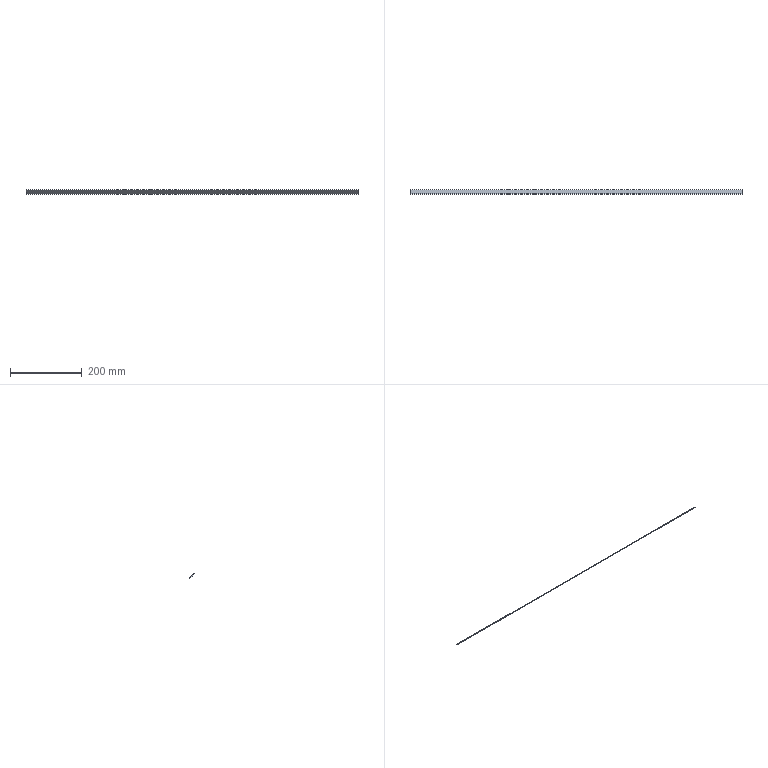Part | SolidWorks | features BaseBody 1 | 1 solid | 6 faces | box 924.6 x 13.8 x 13.8 mm | volume 24987 mm3 | plane 6
STEP:
#1=CARTESIAN_POINT('',(924.6,13.8,2.121));
#2=VERTEX_POINT('',#1);
#3=CARTESIAN_POINT('',(924.6,13.8,0.));
#4=VERTEX_POINT('',#3);
#5=CARTESIAN_POINT('',(924.6,13.8,0.));
#6=DIRECTION('',(0.,0.,-1.));
#7=VECTOR('',#6,1000.);
#8=LINE('',#5,#7);
#9=EDGE_CURVE('',#2,#4,#8,.T.);
#10=ORIENTED_EDGE('',*,*,#9,.T.);
#11=CARTESIAN_POINT('',(0.,13.8,0.));
#12=VERTEX_POINT('',#11);
#13=CARTESIAN_POINT('',(924.6,13.8,0.));
#14=DIRECTION('',(-1.,0.,0.));
#15=VECTOR('',#14,1000.);
#16=LINE('',#13,#15);
#17=EDGE_CURVE('',#4,#12,#16,.T.);
#18=ORIENTED_EDGE('',*,*,#17,.T.);
#19=CARTESIAN_POINT('',(0.,13.8,2.121));
#20=VERTEX_POINT('',#19);
#21=CARTESIAN_POINT('',(0.,13.8,0.));
#22=DIRECTION('',(0.,0.,1.));
#23=VECTOR('',#22,1000.);
#24=LINE('',#21,#23);
#25=EDGE_CURVE('',#12,#20,#24,.T.);
#26=ORIENTED_EDGE('',*,*,#25,.T.);
#27=CARTESIAN_POINT('',(924.6,13.8,2.121));
#28=DIRECTION('',(-1.,0.,0.));
#29=VECTOR('',#28,1000.);
#30=LINE('',#27,#29);
#31=EDGE_CURVE('',#2,#20,#30,.T.);
#32=ORIENTED_EDGE('',*,*,#31,.F.);
#33=EDGE_LOOP('',(#10,#18,#26,#32));
#34=FACE_OUTER_BOUND('',#33,.T.);
#35=CARTESIAN_POINT('',(0.,13.8,0.));
#36=DIRECTION('',(0.,-1.,0.));
#37=DIRECTION('',(0.,0.,-1.));
#38=AXIS2_PLACEMENT_3D('',#35,#36,#37);
#39=PLANE('',#38);
#40=ADVANCED_FACE('',(#34),#39,.F.);
#41=CARTESIAN_POINT('',(0.,0.,13.8));
#42=VERTEX_POINT('',#41);
#43=CARTESIAN_POINT('',(0.,2.121,13.8));
#44=VERTEX_POINT('',#43);
#45=CARTESIAN_POINT('',(0.,0.,13.8));
#46=DIRECTION('',(0.,1.,0.));
#47=VECTOR('',#46,1000.);
#48=LINE('',#45,#47);
#49=EDGE_CURVE('',#42,#44,#48,.T.);
#50=ORIENTED_EDGE('',*,*,#49,.F.);
#51=CARTESIAN_POINT('',(924.6,0.,13.8));
#52=VERTEX_POINT('',#51);
#53=CARTESIAN_POINT('',(924.6,0.,13.8));
#54=DIRECTION('',(-1.,0.,0.));
#55=VECTOR('',#54,1000.);
#56=LINE('',#53,#55);
#57=EDGE_CURVE('',#52,#42,#56,.T.);
#58=ORIENTED_EDGE('',*,*,#57,.F.);
#59=CARTESIAN_POINT('',(924.6,2.121,13.8));
#60=VERTEX_POINT('',#59);
#61=CARTESIAN_POINT('',(924.6,0.,13.8));
#62=DIRECTION('',(0.,1.,0.));
#63=VECTOR('',#62,1000.);
#64=LINE('',#61,#63);
#65=EDGE_CURVE('',#52,#60,#64,.T.);
#66=ORIENTED_EDGE('',*,*,#65,.T.);
#67=CARTESIAN_POINT('',(924.6,2.121,13.8));
#68=DIRECTION('',(1.,0.,0.));
#69=VECTOR('',#68,1000.);
#70=LINE('',#67,#69);
#71=EDGE_CURVE('',#44,#60,#70,.T.);
#72=ORIENTED_EDGE('',*,*,#71,.F.);
#73=EDGE_LOOP('',(#50,#58,#66,#72));
#74=FACE_OUTER_BOUND('',#73,.T.);
#75=CARTESIAN_POINT('',(0.,0.,13.8));
#76=DIRECTION('',(0.,0.,-1.));
#77=DIRECTION('',(0.,-1.,0.));
#78=AXIS2_PLACEMENT_3D('',#75,#76,#77);
#79=PLANE('',#78);
#80=ADVANCED_FACE('',(#74),#79,.F.);
#81=ORIENTED_EDGE('',*,*,#25,.F.);
#82=CARTESIAN_POINT('',(0.,13.8,0.));
#83=DIRECTION('',(0.,-0.7071,0.7071));
#84=VECTOR('',#83,1000.);
#85=LINE('',#82,#84);
#86=EDGE_CURVE('',#12,#42,#85,.T.);
#87=ORIENTED_EDGE('',*,*,#86,.T.);
#88=ORIENTED_EDGE('',*,*,#49,.T.);
#89=CARTESIAN_POINT('',(0.,14.861,1.061));
#90=DIRECTION('',(0.,-0.7071,0.7071));
#91=VECTOR('',#90,1000.);
#92=LINE('',#89,#91);
#93=EDGE_CURVE('',#20,#44,#92,.T.);
#94=ORIENTED_EDGE('',*,*,#93,.F.);
#95=EDGE_LOOP('',(#81,#87,#88,#94));
#96=FACE_OUTER_BOUND('',#95,.T.);
#97=CARTESIAN_POINT('',(0.,0.,0.));
#98=DIRECTION('',(-1.,0.,0.));
#99=DIRECTION('',(0.,0.,1.));
#100=AXIS2_PLACEMENT_3D('',#97,#98,#99);
#101=PLANE('',#100);
#102=ADVANCED_FACE('',(#96),#101,.T.);
#103=CARTESIAN_POINT('',(924.6,13.8,0.));
#104=DIRECTION('',(0.,-0.7071,0.7071));
#105=VECTOR('',#104,1000.);
#106=LINE('',#103,#105);
#107=EDGE_CURVE('',#4,#52,#106,.T.);
#108=ORIENTED_EDGE('',*,*,#107,.F.);
#109=ORIENTED_EDGE('',*,*,#9,.F.);
#110=CARTESIAN_POINT('',(924.6,14.861,1.061));
#111=DIRECTION('',(0.,-0.7071,0.7071));
#112=VECTOR('',#111,1000.);
#113=LINE('',#110,#112);
#114=EDGE_CURVE('',#2,#60,#113,.T.);
#115=ORIENTED_EDGE('',*,*,#114,.T.);
#116=ORIENTED_EDGE('',*,*,#65,.F.);
#117=EDGE_LOOP('',(#108,#109,#115,#116));
#118=FACE_OUTER_BOUND('',#117,.T.);
#119=CARTESIAN_POINT('',(924.6,0.,0.));
#120=DIRECTION('',(-1.,0.,0.));
#121=DIRECTION('',(0.,0.,1.));
#122=AXIS2_PLACEMENT_3D('',#119,#120,#121);
#123=PLANE('',#122);
#124=ADVANCED_FACE('',(#118),#123,.F.);
#125=ORIENTED_EDGE('',*,*,#86,.F.);
#126=ORIENTED_EDGE('',*,*,#17,.F.);
#127=ORIENTED_EDGE('',*,*,#107,.T.);
#128=ORIENTED_EDGE('',*,*,#57,.T.);
#129=EDGE_LOOP('',(#125,#126,#127,#128));
#130=FACE_OUTER_BOUND('',#129,.T.);
#131=CARTESIAN_POINT('',(924.6,13.8,0.));
#132=DIRECTION('',(0.,-0.7071,-0.7071));
#133=DIRECTION('',(0.,-0.7071,0.7071));
#134=AXIS2_PLACEMENT_3D('',#131,#132,#133);
#135=PLANE('',#134);
#136=ADVANCED_FACE('',(#130),#135,.T.);
#137=ORIENTED_EDGE('',*,*,#114,.F.);
#138=ORIENTED_EDGE('',*,*,#31,.T.);
#139=ORIENTED_EDGE('',*,*,#93,.T.);
#140=ORIENTED_EDGE('',*,*,#71,.T.);
#141=EDGE_LOOP('',(#137,#138,#139,#140));
#142=FACE_OUTER_BOUND('',#141,.T.);
#143=CARTESIAN_POINT('',(924.6,14.861,1.061));
#144=DIRECTION('',(0.,-0.7071,-0.7071));
#145=DIRECTION('',(0.,-0.7071,0.7071));
#146=AXIS2_PLACEMENT_3D('',#143,#144,#145);
#147=PLANE('',#146);
#148=ADVANCED_FACE('',(#142),#147,.F.);
#149=CLOSED_SHELL('',(#40,#80,#102,#124,#136,#148));
#150=MANIFOLD_SOLID_BREP('',#149);
#151=CARTESIAN_POINT('',(0.,0.,0.));
#152=DIRECTION('',(0.,0.,1.));
#153=DIRECTION('',(1.,0.,0.));
#154=AXIS2_PLACEMENT_3D('',#151,#152,#153);
#155=(LENGTH_UNIT()NAMED_UNIT(*)SI_UNIT(.MILLI.,.METRE.));
#156=UNCERTAINTY_MEASURE_WITH_UNIT(LENGTH_MEASURE(0.00001),#155,'','');
#157=(NAMED_UNIT(*)PLANE_ANGLE_UNIT()SI_UNIT($,.RADIAN.));
#158=(NAMED_UNIT(*)SI_UNIT($,.STERADIAN.)SOLID_ANGLE_UNIT());
#159=(GEOMETRIC_REPRESENTATION_CONTEXT(3)GLOBAL_UNCERTAINTY_ASSIGNED_CONTEXT((#156))GLOBAL_UNIT_ASSIGNED_CONTEXT((#155,#157,#158))REPRESENTATION_CONTEXT('',''));
#160=ADVANCED_BREP_SHAPE_REPRESENTATION('',(#150,#154),#159);